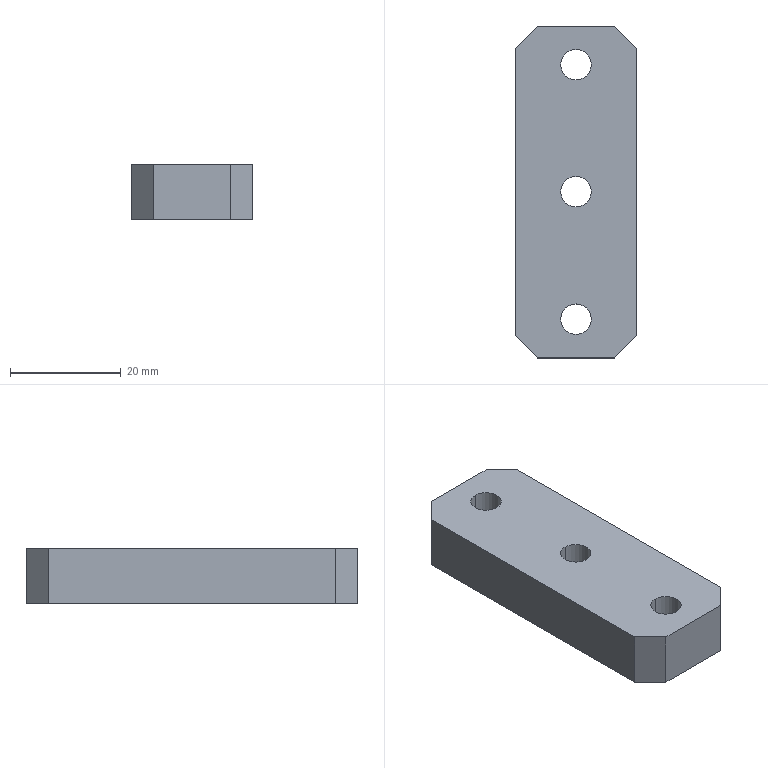Part | Creo | 1 solid | 25 faces | box 22 x 60 x 10 mm | volume 11319 mm3 | plane 13 | cylinder 12 | commonest cylinder face diameters 5.5 x6 9.5 x6
STEP:
#1=CARTESIAN_POINT('',(195.234,-215.142,-294.5));
#2=VERTEX_POINT('',#1);
#3=CARTESIAN_POINT('',(195.234,-163.142,-294.5));
#4=VERTEX_POINT('',#3);
#5=CARTESIAN_POINT('',(195.234,-215.142,-294.5));
#6=DIRECTION('',(0.,1.,0.));
#7=VECTOR('',#6,52.);
#8=LINE('',#5,#7);
#9=EDGE_CURVE('',#2,#4,#8,.T.);
#10=ORIENTED_EDGE('',*,*,#9,.F.);
#11=CARTESIAN_POINT('',(191.234,-219.142,-294.5));
#12=VERTEX_POINT('',#11);
#13=CARTESIAN_POINT('',(191.234,-219.142,-294.5));
#14=DIRECTION('',(0.7071,0.7071,0.));
#15=VECTOR('',#14,5.657);
#16=LINE('',#13,#15);
#17=EDGE_CURVE('',#12,#2,#16,.T.);
#18=ORIENTED_EDGE('',*,*,#17,.F.);
#19=CARTESIAN_POINT('',(177.234,-219.142,-294.5));
#20=VERTEX_POINT('',#19);
#21=CARTESIAN_POINT('',(191.234,-219.142,-294.5));
#22=DIRECTION('',(-1.,0.,0.));
#23=VECTOR('',#22,14.);
#24=LINE('',#21,#23);
#25=EDGE_CURVE('',#12,#20,#24,.T.);
#26=ORIENTED_EDGE('',*,*,#25,.T.);
#27=CARTESIAN_POINT('',(173.234,-215.142,-294.5));
#28=VERTEX_POINT('',#27);
#29=CARTESIAN_POINT('',(173.234,-215.142,-294.5));
#30=DIRECTION('',(0.7071,-0.7071,0.));
#31=VECTOR('',#30,5.657);
#32=LINE('',#29,#31);
#33=EDGE_CURVE('',#28,#20,#32,.T.);
#34=ORIENTED_EDGE('',*,*,#33,.F.);
#35=CARTESIAN_POINT('',(173.234,-163.142,-294.5));
#36=VERTEX_POINT('',#35);
#37=CARTESIAN_POINT('',(173.234,-163.142,-294.5));
#38=DIRECTION('',(0.,-1.,0.));
#39=VECTOR('',#38,52.);
#40=LINE('',#37,#39);
#41=EDGE_CURVE('',#36,#28,#40,.T.);
#42=ORIENTED_EDGE('',*,*,#41,.F.);
#43=CARTESIAN_POINT('',(177.234,-159.142,-294.5));
#44=VERTEX_POINT('',#43);
#45=CARTESIAN_POINT('',(177.234,-159.142,-294.5));
#46=DIRECTION('',(-0.7071,-0.7071,0.));
#47=VECTOR('',#46,5.657);
#48=LINE('',#45,#47);
#49=EDGE_CURVE('',#44,#36,#48,.T.);
#50=ORIENTED_EDGE('',*,*,#49,.F.);
#51=CARTESIAN_POINT('',(191.234,-159.142,-294.5));
#52=VERTEX_POINT('',#51);
#53=CARTESIAN_POINT('',(191.234,-159.142,-294.5));
#54=DIRECTION('',(-1.,0.,0.));
#55=VECTOR('',#54,14.);
#56=LINE('',#53,#55);
#57=EDGE_CURVE('',#52,#44,#56,.T.);
#58=ORIENTED_EDGE('',*,*,#57,.F.);
#59=CARTESIAN_POINT('',(195.234,-163.142,-294.5));
#60=DIRECTION('',(-0.7071,0.7071,0.));
#61=VECTOR('',#60,5.657);
#62=LINE('',#59,#61);
#63=EDGE_CURVE('',#4,#52,#62,.T.);
#64=ORIENTED_EDGE('',*,*,#63,.F.);
#65=EDGE_LOOP('',(#10,#18,#26,#34,#42,#50,#58,#64));
#66=FACE_OUTER_BOUND('',#65,.F.);
#67=CARTESIAN_POINT('',(184.234,-186.342,-294.5));
#68=VERTEX_POINT('',#67);
#69=CARTESIAN_POINT('',(184.234,-191.842,-294.5));
#70=VERTEX_POINT('',#69);
#71=CARTESIAN_POINT('',(184.234,-189.092,-294.5));
#72=DIRECTION('',(0.,0.,-1.));
#73=DIRECTION('',(0.,1.,0.));
#74=AXIS2_PLACEMENT_3D('',#71,#72,#73);
#75=CIRCLE('',#74,2.75);
#76=EDGE_CURVE('',#68,#70,#75,.T.);
#77=ORIENTED_EDGE('',*,*,#76,.F.);
#78=CARTESIAN_POINT('',(184.234,-189.092,-294.5));
#79=DIRECTION('',(0.,0.,-1.));
#80=DIRECTION('',(0.,-1.,0.));
#81=AXIS2_PLACEMENT_3D('',#78,#79,#80);
#82=CIRCLE('',#81,2.75);
#83=EDGE_CURVE('',#70,#68,#82,.T.);
#84=ORIENTED_EDGE('',*,*,#83,.F.);
#85=EDGE_LOOP('',(#77,#84));
#86=FACE_BOUND('',#85,.F.);
#87=CARTESIAN_POINT('',(184.234,-209.392,-294.5));
#88=VERTEX_POINT('',#87);
#89=CARTESIAN_POINT('',(184.234,-214.892,-294.5));
#90=VERTEX_POINT('',#89);
#91=CARTESIAN_POINT('',(184.234,-212.142,-294.5));
#92=DIRECTION('',(0.,0.,-1.));
#93=DIRECTION('',(0.,1.,0.));
#94=AXIS2_PLACEMENT_3D('',#91,#92,#93);
#95=CIRCLE('',#94,2.75);
#96=EDGE_CURVE('',#88,#90,#95,.T.);
#97=ORIENTED_EDGE('',*,*,#96,.F.);
#98=CARTESIAN_POINT('',(184.234,-212.142,-294.5));
#99=DIRECTION('',(0.,0.,-1.));
#100=DIRECTION('',(0.,-1.,0.));
#101=AXIS2_PLACEMENT_3D('',#98,#99,#100);
#102=CIRCLE('',#101,2.75);
#103=EDGE_CURVE('',#90,#88,#102,.T.);
#104=ORIENTED_EDGE('',*,*,#103,.F.);
#105=EDGE_LOOP('',(#97,#104));
#106=FACE_BOUND('',#105,.F.);
#107=CARTESIAN_POINT('',(184.234,-163.392,-294.5));
#108=VERTEX_POINT('',#107);
#109=CARTESIAN_POINT('',(184.234,-168.892,-294.5));
#110=VERTEX_POINT('',#109);
#111=CARTESIAN_POINT('',(184.234,-166.142,-294.5));
#112=DIRECTION('',(0.,0.,-1.));
#113=DIRECTION('',(0.,1.,0.));
#114=AXIS2_PLACEMENT_3D('',#111,#112,#113);
#115=CIRCLE('',#114,2.75);
#116=EDGE_CURVE('',#108,#110,#115,.T.);
#117=ORIENTED_EDGE('',*,*,#116,.F.);
#118=CARTESIAN_POINT('',(184.234,-166.142,-294.5));
#119=DIRECTION('',(0.,0.,-1.));
#120=DIRECTION('',(0.,-1.,0.));
#121=AXIS2_PLACEMENT_3D('',#118,#119,#120);
#122=CIRCLE('',#121,2.75);
#123=EDGE_CURVE('',#110,#108,#122,.T.);
#124=ORIENTED_EDGE('',*,*,#123,.F.);
#125=EDGE_LOOP('',(#117,#124));
#126=FACE_BOUND('',#125,.F.);
#127=CARTESIAN_POINT('',(174.234,-195.192,-294.5));
#128=DIRECTION('',(0.,0.,1.));
#129=DIRECTION('',(0.,-1.,0.));
#130=AXIS2_PLACEMENT_3D('',#127,#128,#129);
#131=PLANE('',#130);
#132=ADVANCED_FACE('',(#66,#86,#106,#126),#131,.T.);
#133=CARTESIAN_POINT('',(195.234,-163.142,-304.5));
#134=VERTEX_POINT('',#133);
#135=CARTESIAN_POINT('',(195.234,-215.142,-304.5));
#136=VERTEX_POINT('',#135);
#137=CARTESIAN_POINT('',(195.234,-163.142,-304.5));
#138=DIRECTION('',(0.,-1.,0.));
#139=VECTOR('',#138,52.);
#140=LINE('',#137,#139);
#141=EDGE_CURVE('',#134,#136,#140,.T.);
#142=ORIENTED_EDGE('',*,*,#141,.T.);
#143=CARTESIAN_POINT('',(195.234,-215.142,-294.5));
#144=DIRECTION('',(0.,0.,-1.));
#145=VECTOR('',#144,10.);
#146=LINE('',#143,#145);
#147=EDGE_CURVE('',#2,#136,#146,.T.);
#148=ORIENTED_EDGE('',*,*,#147,.F.);
#149=ORIENTED_EDGE('',*,*,#9,.T.);
#150=CARTESIAN_POINT('',(195.234,-163.142,-304.5));
#151=DIRECTION('',(0.,0.,1.));
#152=VECTOR('',#151,10.);
#153=LINE('',#150,#152);
#154=EDGE_CURVE('',#134,#4,#153,.T.);
#155=ORIENTED_EDGE('',*,*,#154,.F.);
#156=EDGE_LOOP('',(#142,#148,#149,#155));
#157=FACE_OUTER_BOUND('',#156,.F.);
#158=CARTESIAN_POINT('',(195.234,-212.942,-299.5));
#159=DIRECTION('',(-1.,0.,0.));
#160=DIRECTION('',(0.,0.,1.));
#161=AXIS2_PLACEMENT_3D('',#158,#159,#160);
#162=PLANE('',#161);
#163=ADVANCED_FACE('',(#157),#162,.F.);
#164=CARTESIAN_POINT('',(173.234,-215.142,-304.5));
#165=VERTEX_POINT('',#164);
#166=CARTESIAN_POINT('',(173.234,-163.142,-304.5));
#167=VERTEX_POINT('',#166);
#168=CARTESIAN_POINT('',(173.234,-215.142,-304.5));
#169=DIRECTION('',(0.,1.,0.));
#170=VECTOR('',#169,52.);
#171=LINE('',#168,#170);
#172=EDGE_CURVE('',#165,#167,#171,.T.);
#173=ORIENTED_EDGE('',*,*,#172,.F.);
#174=CARTESIAN_POINT('',(177.234,-219.142,-304.5));
#175=VERTEX_POINT('',#174);
#176=CARTESIAN_POINT('',(177.234,-219.142,-304.5));
#177=DIRECTION('',(-0.7071,0.7071,0.));
#178=VECTOR('',#177,5.657);
#179=LINE('',#176,#178);
#180=EDGE_CURVE('',#175,#165,#179,.T.);
#181=ORIENTED_EDGE('',*,*,#180,.F.);
#182=CARTESIAN_POINT('',(191.234,-219.142,-304.5));
#183=VERTEX_POINT('',#182);
#184=CARTESIAN_POINT('',(177.234,-219.142,-304.5));
#185=DIRECTION('',(1.,0.,0.));
#186=VECTOR('',#185,14.);
#187=LINE('',#184,#186);
#188=EDGE_CURVE('',#175,#183,#187,.T.);
#189=ORIENTED_EDGE('',*,*,#188,.T.);
#190=CARTESIAN_POINT('',(195.234,-215.142,-304.5));
#191=DIRECTION('',(-0.7071,-0.7071,0.));
#192=VECTOR('',#191,5.657);
#193=LINE('',#190,#192);
#194=EDGE_CURVE('',#136,#183,#193,.T.);
#195=ORIENTED_EDGE('',*,*,#194,.F.);
#196=ORIENTED_EDGE('',*,*,#141,.F.);
#197=CARTESIAN_POINT('',(191.234,-159.142,-304.5));
#198=VERTEX_POINT('',#197);
#199=CARTESIAN_POINT('',(191.234,-159.142,-304.5));
#200=DIRECTION('',(0.7071,-0.7071,0.));
#201=VECTOR('',#200,5.657);
#202=LINE('',#199,#201);
#203=EDGE_CURVE('',#198,#134,#202,.T.);
#204=ORIENTED_EDGE('',*,*,#203,.F.);
#205=CARTESIAN_POINT('',(177.234,-159.142,-304.5));
#206=VERTEX_POINT('',#205);
#207=CARTESIAN_POINT('',(177.234,-159.142,-304.5));
#208=DIRECTION('',(1.,0.,0.));
#209=VECTOR('',#208,14.);
#210=LINE('',#207,#209);
#211=EDGE_CURVE('',#206,#198,#210,.T.);
#212=ORIENTED_EDGE('',*,*,#211,.F.);
#213=CARTESIAN_POINT('',(173.234,-163.142,-304.5));
#214=DIRECTION('',(0.7071,0.7071,0.));
#215=VECTOR('',#214,5.657);
#216=LINE('',#213,#215);
#217=EDGE_CURVE('',#167,#206,#216,.T.);
#218=ORIENTED_EDGE('',*,*,#217,.F.);
#219=EDGE_LOOP('',(#173,#181,#189,#195,#196,#204,#212,#218));
#220=FACE_OUTER_BOUND('',#219,.F.);
#221=CARTESIAN_POINT('',(184.234,-184.342,-304.5));
#222=VERTEX_POINT('',#221);
#223=CARTESIAN_POINT('',(184.234,-193.842,-304.5));
#224=VERTEX_POINT('',#223);
#225=CARTESIAN_POINT('',(184.234,-189.092,-304.5));
#226=DIRECTION('',(0.,0.,1.));
#227=DIRECTION('',(0.,1.,0.));
#228=AXIS2_PLACEMENT_3D('',#225,#226,#227);
#229=CIRCLE('',#228,4.75);
#230=EDGE_CURVE('',#222,#224,#229,.T.);
#231=ORIENTED_EDGE('',*,*,#230,.F.);
#232=CARTESIAN_POINT('',(184.234,-189.092,-304.5));
#233=DIRECTION('',(0.,0.,1.));
#234=DIRECTION('',(0.,-1.,0.));
#235=AXIS2_PLACEMENT_3D('',#232,#233,#234);
#236=CIRCLE('',#235,4.75);
#237=EDGE_CURVE('',#224,#222,#236,.T.);
#238=ORIENTED_EDGE('',*,*,#237,.F.);
#239=EDGE_LOOP('',(#231,#238));
#240=FACE_BOUND('',#239,.F.);
#241=CARTESIAN_POINT('',(184.234,-207.392,-304.5));
#242=VERTEX_POINT('',#241);
#243=CARTESIAN_POINT('',(184.234,-216.892,-304.5));
#244=VERTEX_POINT('',#243);
#245=CARTESIAN_POINT('',(184.234,-212.142,-304.5));
#246=DIRECTION('',(0.,0.,1.));
#247=DIRECTION('',(0.,1.,0.));
#248=AXIS2_PLACEMENT_3D('',#245,#246,#247);
#249=CIRCLE('',#248,4.75);
#250=EDGE_CURVE('',#242,#244,#249,.T.);
#251=ORIENTED_EDGE('',*,*,#250,.F.);
#252=CARTESIAN_POINT('',(184.234,-212.142,-304.5));
#253=DIRECTION('',(0.,0.,1.));
#254=DIRECTION('',(0.,-1.,0.));
#255=AXIS2_PLACEMENT_3D('',#252,#253,#254);
#256=CIRCLE('',#255,4.75);
#257=EDGE_CURVE('',#244,#242,#256,.T.);
#258=ORIENTED_EDGE('',*,*,#257,.F.);
#259=EDGE_LOOP('',(#251,#258));
#260=FACE_BOUND('',#259,.F.);
#261=CARTESIAN_POINT('',(184.234,-161.392,-304.5));
#262=VERTEX_POINT('',#261);
#263=CARTESIAN_POINT('',(184.234,-170.892,-304.5));
#264=VERTEX_POINT('',#263);
#265=CARTESIAN_POINT('',(184.234,-166.142,-304.5));
#266=DIRECTION('',(0.,0.,1.));
#267=DIRECTION('',(0.,1.,0.));
#268=AXIS2_PLACEMENT_3D('',#265,#266,#267);
#269=CIRCLE('',#268,4.75);
#270=EDGE_CURVE('',#262,#264,#269,.T.);
#271=ORIENTED_EDGE('',*,*,#270,.F.);
#272=CARTESIAN_POINT('',(184.234,-166.142,-304.5));
#273=DIRECTION('',(0.,0.,1.));
#274=DIRECTION('',(0.,-1.,0.));
#275=AXIS2_PLACEMENT_3D('',#272,#273,#274);
#276=CIRCLE('',#275,4.75);
#277=EDGE_CURVE('',#264,#262,#276,.T.);
#278=ORIENTED_EDGE('',*,*,#277,.F.);
#279=EDGE_LOOP('',(#271,#278));
#280=FACE_BOUND('',#279,.F.);
#281=CARTESIAN_POINT('',(174.234,-195.192,-304.5));
#282=DIRECTION('',(0.,0.,-1.));
#283=DIRECTION('',(0.,1.,0.));
#284=AXIS2_PLACEMENT_3D('',#281,#282,#283);
#285=PLANE('',#284);
#286=ADVANCED_FACE('',(#220,#240,#260,#280),#285,.T.);
#287=ORIENTED_EDGE('',*,*,#41,.T.);
#288=CARTESIAN_POINT('',(173.234,-215.142,-304.5));
#289=DIRECTION('',(0.,0.,1.));
#290=VECTOR('',#289,10.);
#291=LINE('',#288,#290);
#292=EDGE_CURVE('',#165,#28,#291,.T.);
#293=ORIENTED_EDGE('',*,*,#292,.F.);
#294=ORIENTED_EDGE('',*,*,#172,.T.);
#295=CARTESIAN_POINT('',(173.234,-163.142,-294.5));
#296=DIRECTION('',(0.,0.,-1.));
#297=VECTOR('',#296,10.);
#298=LINE('',#295,#297);
#299=EDGE_CURVE('',#36,#167,#298,.T.);
#300=ORIENTED_EDGE('',*,*,#299,.F.);
#301=EDGE_LOOP('',(#287,#293,#294,#300));
#302=FACE_OUTER_BOUND('',#301,.F.);
#303=CARTESIAN_POINT('',(173.234,-190.442,-299.5));
#304=DIRECTION('',(1.,0.,0.));
#305=DIRECTION('',(0.,0.,1.));
#306=AXIS2_PLACEMENT_3D('',#303,#304,#305);
#307=PLANE('',#306);
#308=ADVANCED_FACE('',(#302),#307,.F.);
#309=ORIENTED_EDGE('',*,*,#180,.T.);
#310=ORIENTED_EDGE('',*,*,#292,.T.);
#311=ORIENTED_EDGE('',*,*,#33,.T.);
#312=CARTESIAN_POINT('',(177.234,-219.142,-294.5));
#313=DIRECTION('',(0.,0.,-1.));
#314=VECTOR('',#313,10.);
#315=LINE('',#312,#314);
#316=EDGE_CURVE('',#20,#175,#315,.T.);
#317=ORIENTED_EDGE('',*,*,#316,.T.);
#318=EDGE_LOOP('',(#309,#310,#311,#317));
#319=FACE_OUTER_BOUND('',#318,.F.);
#320=CARTESIAN_POINT('',(177.234,-219.142,-299.5));
#321=DIRECTION('',(0.7071,0.7071,0.));
#322=DIRECTION('',(0.7071,-0.7071,0.));
#323=AXIS2_PLACEMENT_3D('',#320,#321,#322);
#324=PLANE('',#323);
#325=ADVANCED_FACE('',(#319),#324,.F.);
#326=ORIENTED_EDGE('',*,*,#25,.F.);
#327=CARTESIAN_POINT('',(191.234,-219.142,-304.5));
#328=DIRECTION('',(0.,0.,1.));
#329=VECTOR('',#328,10.);
#330=LINE('',#327,#329);
#331=EDGE_CURVE('',#183,#12,#330,.T.);
#332=ORIENTED_EDGE('',*,*,#331,.F.);
#333=ORIENTED_EDGE('',*,*,#188,.F.);
#334=ORIENTED_EDGE('',*,*,#316,.F.);
#335=EDGE_LOOP('',(#326,#332,#333,#334));
#336=FACE_OUTER_BOUND('',#335,.F.);
#337=CARTESIAN_POINT('',(172.234,-219.142,-299.5));
#338=DIRECTION('',(0.,1.,0.));
#339=DIRECTION('',(0.,0.,-1.));
#340=AXIS2_PLACEMENT_3D('',#337,#338,#339);
#341=PLANE('',#340);
#342=ADVANCED_FACE('',(#336),#341,.F.);
#343=ORIENTED_EDGE('',*,*,#194,.T.);
#344=ORIENTED_EDGE('',*,*,#331,.T.);
#345=ORIENTED_EDGE('',*,*,#17,.T.);
#346=ORIENTED_EDGE('',*,*,#147,.T.);
#347=EDGE_LOOP('',(#343,#344,#345,#346));
#348=FACE_OUTER_BOUND('',#347,.F.);
#349=CARTESIAN_POINT('',(195.234,-215.142,-299.5));
#350=DIRECTION('',(-0.7071,0.7071,0.));
#351=DIRECTION('',(0.7071,0.7071,0.));
#352=AXIS2_PLACEMENT_3D('',#349,#350,#351);
#353=PLANE('',#352);
#354=ADVANCED_FACE('',(#348),#353,.F.);
#355=ORIENTED_EDGE('',*,*,#217,.T.);
#356=CARTESIAN_POINT('',(177.234,-159.142,-304.5));
#357=DIRECTION('',(0.,0.,1.));
#358=VECTOR('',#357,10.);
#359=LINE('',#356,#358);
#360=EDGE_CURVE('',#206,#44,#359,.T.);
#361=ORIENTED_EDGE('',*,*,#360,.T.);
#362=ORIENTED_EDGE('',*,*,#49,.T.);
#363=ORIENTED_EDGE('',*,*,#299,.T.);
#364=EDGE_LOOP('',(#355,#361,#362,#363));
#365=FACE_OUTER_BOUND('',#364,.F.);
#366=CARTESIAN_POINT('',(173.234,-163.142,-299.5));
#367=DIRECTION('',(0.7071,-0.7071,0.));
#368=DIRECTION('',(-0.7071,-0.7071,0.));
#369=AXIS2_PLACEMENT_3D('',#366,#367,#368);
#370=PLANE('',#369);
#371=ADVANCED_FACE('',(#365),#370,.F.);
#372=ORIENTED_EDGE('',*,*,#57,.T.);
#373=ORIENTED_EDGE('',*,*,#360,.F.);
#374=ORIENTED_EDGE('',*,*,#211,.T.);
#375=CARTESIAN_POINT('',(191.234,-159.142,-294.5));
#376=DIRECTION('',(0.,0.,-1.));
#377=VECTOR('',#376,10.);
#378=LINE('',#375,#377);
#379=EDGE_CURVE('',#52,#198,#378,.T.);
#380=ORIENTED_EDGE('',*,*,#379,.F.);
#381=EDGE_LOOP('',(#372,#373,#374,#380));
#382=FACE_OUTER_BOUND('',#381,.F.);
#383=CARTESIAN_POINT('',(172.234,-159.142,-299.5));
#384=DIRECTION('',(0.,-1.,0.));
#385=DIRECTION('',(0.,0.,-1.));
#386=AXIS2_PLACEMENT_3D('',#383,#384,#385);
#387=PLANE('',#386);
#388=ADVANCED_FACE('',(#382),#387,.F.);
#389=ORIENTED_EDGE('',*,*,#203,.T.);
#390=ORIENTED_EDGE('',*,*,#154,.T.);
#391=ORIENTED_EDGE('',*,*,#63,.T.);
#392=ORIENTED_EDGE('',*,*,#379,.T.);
#393=EDGE_LOOP('',(#389,#390,#391,#392));
#394=FACE_OUTER_BOUND('',#393,.F.);
#395=CARTESIAN_POINT('',(191.234,-159.142,-299.5));
#396=DIRECTION('',(-0.7071,-0.7071,0.));
#397=DIRECTION('',(-0.7071,0.7071,0.));
#398=AXIS2_PLACEMENT_3D('',#395,#396,#397);
#399=PLANE('',#398);
#400=ADVANCED_FACE('',(#394),#399,.F.);
#401=ORIENTED_EDGE('',*,*,#230,.T.);
#402=CARTESIAN_POINT('',(184.234,-193.842,-298.5));
#403=VERTEX_POINT('',#402);
#404=CARTESIAN_POINT('',(184.234,-193.842,-298.5));
#405=DIRECTION('',(0.,0.,-1.));
#406=VECTOR('',#405,6.);
#407=LINE('',#404,#406);
#408=EDGE_CURVE('',#403,#224,#407,.T.);
#409=ORIENTED_EDGE('',*,*,#408,.F.);
#410=CARTESIAN_POINT('',(184.234,-184.342,-298.5));
#411=VERTEX_POINT('',#410);
#412=CARTESIAN_POINT('',(184.234,-189.092,-298.5));
#413=DIRECTION('',(0.,0.,-1.));
#414=DIRECTION('',(0.,-1.,0.));
#415=AXIS2_PLACEMENT_3D('',#412,#413,#414);
#416=CIRCLE('',#415,4.75);
#417=EDGE_CURVE('',#403,#411,#416,.T.);
#418=ORIENTED_EDGE('',*,*,#417,.T.);
#419=CARTESIAN_POINT('',(184.234,-184.342,-298.5));
#420=DIRECTION('',(0.,0.,-1.));
#421=VECTOR('',#420,6.);
#422=LINE('',#419,#421);
#423=EDGE_CURVE('',#411,#222,#422,.T.);
#424=ORIENTED_EDGE('',*,*,#423,.T.);
#425=EDGE_LOOP('',(#401,#409,#418,#424));
#426=FACE_OUTER_BOUND('',#425,.F.);
#427=CARTESIAN_POINT('',(184.234,-189.092,-298.5));
#428=DIRECTION('',(0.,0.,-1.));
#429=DIRECTION('',(0.,1.,0.));
#430=AXIS2_PLACEMENT_3D('',#427,#428,#429);
#431=CYLINDRICAL_SURFACE('',#430,4.75);
#432=ADVANCED_FACE('',(#426),#431,.F.);
#433=ORIENTED_EDGE('',*,*,#237,.T.);
#434=ORIENTED_EDGE('',*,*,#423,.F.);
#435=CARTESIAN_POINT('',(184.234,-189.092,-298.5));
#436=DIRECTION('',(0.,0.,-1.));
#437=DIRECTION('',(0.,1.,0.));
#438=AXIS2_PLACEMENT_3D('',#435,#436,#437);
#439=CIRCLE('',#438,4.75);
#440=EDGE_CURVE('',#411,#403,#439,.T.);
#441=ORIENTED_EDGE('',*,*,#440,.T.);
#442=ORIENTED_EDGE('',*,*,#408,.T.);
#443=EDGE_LOOP('',(#433,#434,#441,#442));
#444=FACE_OUTER_BOUND('',#443,.F.);
#445=CARTESIAN_POINT('',(184.234,-189.092,-298.5));
#446=DIRECTION('',(0.,0.,-1.));
#447=DIRECTION('',(0.,1.,0.));
#448=AXIS2_PLACEMENT_3D('',#445,#446,#447);
#449=CYLINDRICAL_SURFACE('',#448,4.75);
#450=ADVANCED_FACE('',(#444),#449,.F.);
#451=ORIENTED_EDGE('',*,*,#440,.F.);
#452=ORIENTED_EDGE('',*,*,#417,.F.);
#453=EDGE_LOOP('',(#451,#452));
#454=FACE_OUTER_BOUND('',#453,.F.);
#455=CARTESIAN_POINT('',(184.234,-186.342,-298.5));
#456=VERTEX_POINT('',#455);
#457=CARTESIAN_POINT('',(184.234,-191.842,-298.5));
#458=VERTEX_POINT('',#457);
#459=CARTESIAN_POINT('',(184.234,-189.092,-298.5));
#460=DIRECTION('',(0.,0.,1.));
#461=DIRECTION('',(0.,1.,0.));
#462=AXIS2_PLACEMENT_3D('',#459,#460,#461);
#463=CIRCLE('',#462,2.75);
#464=EDGE_CURVE('',#456,#458,#463,.T.);
#465=ORIENTED_EDGE('',*,*,#464,.F.);
#466=CARTESIAN_POINT('',(184.234,-189.092,-298.5));
#467=DIRECTION('',(0.,0.,1.));
#468=DIRECTION('',(0.,-1.,0.));
#469=AXIS2_PLACEMENT_3D('',#466,#467,#468);
#470=CIRCLE('',#469,2.75);
#471=EDGE_CURVE('',#458,#456,#470,.T.);
#472=ORIENTED_EDGE('',*,*,#471,.F.);
#473=EDGE_LOOP('',(#465,#472));
#474=FACE_BOUND('',#473,.F.);
#475=CARTESIAN_POINT('',(184.234,-189.092,-298.5));
#476=DIRECTION('',(0.,0.,1.));
#477=DIRECTION('',(0.,-1.,0.));
#478=AXIS2_PLACEMENT_3D('',#475,#476,#477);
#479=PLANE('',#478);
#480=ADVANCED_FACE('',(#454,#474),#479,.F.);
#481=ORIENTED_EDGE('',*,*,#464,.T.);
#482=CARTESIAN_POINT('',(184.234,-191.842,-294.5));
#483=DIRECTION('',(0.,0.,-1.));
#484=VECTOR('',#483,4.);
#485=LINE('',#482,#484);
#486=EDGE_CURVE('',#70,#458,#485,.T.);
#487=ORIENTED_EDGE('',*,*,#486,.F.);
#488=ORIENTED_EDGE('',*,*,#83,.T.);
#489=CARTESIAN_POINT('',(184.234,-186.342,-294.5));
#490=DIRECTION('',(0.,0.,-1.));
#491=VECTOR('',#490,4.);
#492=LINE('',#489,#491);
#493=EDGE_CURVE('',#68,#456,#492,.T.);
#494=ORIENTED_EDGE('',*,*,#493,.T.);
#495=EDGE_LOOP('',(#481,#487,#488,#494));
#496=FACE_OUTER_BOUND('',#495,.F.);
#497=CARTESIAN_POINT('',(184.234,-189.092,-294.5));
#498=DIRECTION('',(0.,0.,-1.));
#499=DIRECTION('',(0.,1.,0.));
#500=AXIS2_PLACEMENT_3D('',#497,#498,#499);
#501=CYLINDRICAL_SURFACE('',#500,2.75);
#502=ADVANCED_FACE('',(#496),#501,.F.);
#503=ORIENTED_EDGE('',*,*,#471,.T.);
#504=ORIENTED_EDGE('',*,*,#493,.F.);
#505=ORIENTED_EDGE('',*,*,#76,.T.);
#506=ORIENTED_EDGE('',*,*,#486,.T.);
#507=EDGE_LOOP('',(#503,#504,#505,#506));
#508=FACE_OUTER_BOUND('',#507,.F.);
#509=CARTESIAN_POINT('',(184.234,-189.092,-294.5));
#510=DIRECTION('',(0.,0.,-1.));
#511=DIRECTION('',(0.,1.,0.));
#512=AXIS2_PLACEMENT_3D('',#509,#510,#511);
#513=CYLINDRICAL_SURFACE('',#512,2.75);
#514=ADVANCED_FACE('',(#508),#513,.F.);
#515=ORIENTED_EDGE('',*,*,#250,.T.);
#516=CARTESIAN_POINT('',(184.234,-216.892,-298.5));
#517=VERTEX_POINT('',#516);
#518=CARTESIAN_POINT('',(184.234,-216.892,-298.5));
#519=DIRECTION('',(0.,0.,-1.));
#520=VECTOR('',#519,6.);
#521=LINE('',#518,#520);
#522=EDGE_CURVE('',#517,#244,#521,.T.);
#523=ORIENTED_EDGE('',*,*,#522,.F.);
#524=CARTESIAN_POINT('',(184.234,-207.392,-298.5));
#525=VERTEX_POINT('',#524);
#526=CARTESIAN_POINT('',(184.234,-212.142,-298.5));
#527=DIRECTION('',(0.,0.,-1.));
#528=DIRECTION('',(0.,-1.,0.));
#529=AXIS2_PLACEMENT_3D('',#526,#527,#528);
#530=CIRCLE('',#529,4.75);
#531=EDGE_CURVE('',#517,#525,#530,.T.);
#532=ORIENTED_EDGE('',*,*,#531,.T.);
#533=CARTESIAN_POINT('',(184.234,-207.392,-298.5));
#534=DIRECTION('',(0.,0.,-1.));
#535=VECTOR('',#534,6.);
#536=LINE('',#533,#535);
#537=EDGE_CURVE('',#525,#242,#536,.T.);
#538=ORIENTED_EDGE('',*,*,#537,.T.);
#539=EDGE_LOOP('',(#515,#523,#532,#538));
#540=FACE_OUTER_BOUND('',#539,.F.);
#541=CARTESIAN_POINT('',(184.234,-212.142,-298.5));
#542=DIRECTION('',(0.,0.,-1.));
#543=DIRECTION('',(0.,1.,0.));
#544=AXIS2_PLACEMENT_3D('',#541,#542,#543);
#545=CYLINDRICAL_SURFACE('',#544,4.75);
#546=ADVANCED_FACE('',(#540),#545,.F.);
#547=ORIENTED_EDGE('',*,*,#257,.T.);
#548=ORIENTED_EDGE('',*,*,#537,.F.);
#549=CARTESIAN_POINT('',(184.234,-212.142,-298.5));
#550=DIRECTION('',(0.,0.,-1.));
#551=DIRECTION('',(0.,1.,0.));
#552=AXIS2_PLACEMENT_3D('',#549,#550,#551);
#553=CIRCLE('',#552,4.75);
#554=EDGE_CURVE('',#525,#517,#553,.T.);
#555=ORIENTED_EDGE('',*,*,#554,.T.);
#556=ORIENTED_EDGE('',*,*,#522,.T.);
#557=EDGE_LOOP('',(#547,#548,#555,#556));
#558=FACE_OUTER_BOUND('',#557,.F.);
#559=CARTESIAN_POINT('',(184.234,-212.142,-298.5));
#560=DIRECTION('',(0.,0.,-1.));
#561=DIRECTION('',(0.,1.,0.));
#562=AXIS2_PLACEMENT_3D('',#559,#560,#561);
#563=CYLINDRICAL_SURFACE('',#562,4.75);
#564=ADVANCED_FACE('',(#558),#563,.F.);
#565=ORIENTED_EDGE('',*,*,#554,.F.);
#566=ORIENTED_EDGE('',*,*,#531,.F.);
#567=EDGE_LOOP('',(#565,#566));
#568=FACE_OUTER_BOUND('',#567,.F.);
#569=CARTESIAN_POINT('',(184.234,-209.392,-298.5));
#570=VERTEX_POINT('',#569);
#571=CARTESIAN_POINT('',(184.234,-214.892,-298.5));
#572=VERTEX_POINT('',#571);
#573=CARTESIAN_POINT('',(184.234,-212.142,-298.5));
#574=DIRECTION('',(0.,0.,1.));
#575=DIRECTION('',(0.,1.,0.));
#576=AXIS2_PLACEMENT_3D('',#573,#574,#575);
#577=CIRCLE('',#576,2.75);
#578=EDGE_CURVE('',#570,#572,#577,.T.);
#579=ORIENTED_EDGE('',*,*,#578,.F.);
#580=CARTESIAN_POINT('',(184.234,-212.142,-298.5));
#581=DIRECTION('',(0.,0.,1.));
#582=DIRECTION('',(0.,-1.,0.));
#583=AXIS2_PLACEMENT_3D('',#580,#581,#582);
#584=CIRCLE('',#583,2.75);
#585=EDGE_CURVE('',#572,#570,#584,.T.);
#586=ORIENTED_EDGE('',*,*,#585,.F.);
#587=EDGE_LOOP('',(#579,#586));
#588=FACE_BOUND('',#587,.F.);
#589=CARTESIAN_POINT('',(184.234,-212.142,-298.5));
#590=DIRECTION('',(0.,0.,1.));
#591=DIRECTION('',(0.,-1.,0.));
#592=AXIS2_PLACEMENT_3D('',#589,#590,#591);
#593=PLANE('',#592);
#594=ADVANCED_FACE('',(#568,#588),#593,.F.);
#595=ORIENTED_EDGE('',*,*,#578,.T.);
#596=CARTESIAN_POINT('',(184.234,-214.892,-294.5));
#597=DIRECTION('',(0.,0.,-1.));
#598=VECTOR('',#597,4.);
#599=LINE('',#596,#598);
#600=EDGE_CURVE('',#90,#572,#599,.T.);
#601=ORIENTED_EDGE('',*,*,#600,.F.);
#602=ORIENTED_EDGE('',*,*,#103,.T.);
#603=CARTESIAN_POINT('',(184.234,-209.392,-294.5));
#604=DIRECTION('',(0.,0.,-1.));
#605=VECTOR('',#604,4.);
#606=LINE('',#603,#605);
#607=EDGE_CURVE('',#88,#570,#606,.T.);
#608=ORIENTED_EDGE('',*,*,#607,.T.);
#609=EDGE_LOOP('',(#595,#601,#602,#608));
#610=FACE_OUTER_BOUND('',#609,.F.);
#611=CARTESIAN_POINT('',(184.234,-212.142,-294.5));
#612=DIRECTION('',(0.,0.,-1.));
#613=DIRECTION('',(0.,1.,0.));
#614=AXIS2_PLACEMENT_3D('',#611,#612,#613);
#615=CYLINDRICAL_SURFACE('',#614,2.75);
#616=ADVANCED_FACE('',(#610),#615,.F.);
#617=ORIENTED_EDGE('',*,*,#585,.T.);
#618=ORIENTED_EDGE('',*,*,#607,.F.);
#619=ORIENTED_EDGE('',*,*,#96,.T.);
#620=ORIENTED_EDGE('',*,*,#600,.T.);
#621=EDGE_LOOP('',(#617,#618,#619,#620));
#622=FACE_OUTER_BOUND('',#621,.F.);
#623=CARTESIAN_POINT('',(184.234,-212.142,-294.5));
#624=DIRECTION('',(0.,0.,-1.));
#625=DIRECTION('',(0.,1.,0.));
#626=AXIS2_PLACEMENT_3D('',#623,#624,#625);
#627=CYLINDRICAL_SURFACE('',#626,2.75);
#628=ADVANCED_FACE('',(#622),#627,.F.);
#629=ORIENTED_EDGE('',*,*,#270,.T.);
#630=CARTESIAN_POINT('',(184.234,-170.892,-298.5));
#631=VERTEX_POINT('',#630);
#632=CARTESIAN_POINT('',(184.234,-170.892,-298.5));
#633=DIRECTION('',(0.,0.,-1.));
#634=VECTOR('',#633,6.);
#635=LINE('',#632,#634);
#636=EDGE_CURVE('',#631,#264,#635,.T.);
#637=ORIENTED_EDGE('',*,*,#636,.F.);
#638=CARTESIAN_POINT('',(184.234,-161.392,-298.5));
#639=VERTEX_POINT('',#638);
#640=CARTESIAN_POINT('',(184.234,-166.142,-298.5));
#641=DIRECTION('',(0.,0.,-1.));
#642=DIRECTION('',(0.,-1.,0.));
#643=AXIS2_PLACEMENT_3D('',#640,#641,#642);
#644=CIRCLE('',#643,4.75);
#645=EDGE_CURVE('',#631,#639,#644,.T.);
#646=ORIENTED_EDGE('',*,*,#645,.T.);
#647=CARTESIAN_POINT('',(184.234,-161.392,-298.5));
#648=DIRECTION('',(0.,0.,-1.));
#649=VECTOR('',#648,6.);
#650=LINE('',#647,#649);
#651=EDGE_CURVE('',#639,#262,#650,.T.);
#652=ORIENTED_EDGE('',*,*,#651,.T.);
#653=EDGE_LOOP('',(#629,#637,#646,#652));
#654=FACE_OUTER_BOUND('',#653,.F.);
#655=CARTESIAN_POINT('',(184.234,-166.142,-298.5));
#656=DIRECTION('',(0.,0.,-1.));
#657=DIRECTION('',(0.,1.,0.));
#658=AXIS2_PLACEMENT_3D('',#655,#656,#657);
#659=CYLINDRICAL_SURFACE('',#658,4.75);
#660=ADVANCED_FACE('',(#654),#659,.F.);
#661=ORIENTED_EDGE('',*,*,#277,.T.);
#662=ORIENTED_EDGE('',*,*,#651,.F.);
#663=CARTESIAN_POINT('',(184.234,-166.142,-298.5));
#664=DIRECTION('',(0.,0.,-1.));
#665=DIRECTION('',(0.,1.,0.));
#666=AXIS2_PLACEMENT_3D('',#663,#664,#665);
#667=CIRCLE('',#666,4.75);
#668=EDGE_CURVE('',#639,#631,#667,.T.);
#669=ORIENTED_EDGE('',*,*,#668,.T.);
#670=ORIENTED_EDGE('',*,*,#636,.T.);
#671=EDGE_LOOP('',(#661,#662,#669,#670));
#672=FACE_OUTER_BOUND('',#671,.F.);
#673=CARTESIAN_POINT('',(184.234,-166.142,-298.5));
#674=DIRECTION('',(0.,0.,-1.));
#675=DIRECTION('',(0.,1.,0.));
#676=AXIS2_PLACEMENT_3D('',#673,#674,#675);
#677=CYLINDRICAL_SURFACE('',#676,4.75);
#678=ADVANCED_FACE('',(#672),#677,.F.);
#679=ORIENTED_EDGE('',*,*,#668,.F.);
#680=ORIENTED_EDGE('',*,*,#645,.F.);
#681=EDGE_LOOP('',(#679,#680));
#682=FACE_OUTER_BOUND('',#681,.F.);
#683=CARTESIAN_POINT('',(184.234,-163.392,-298.5));
#684=VERTEX_POINT('',#683);
#685=CARTESIAN_POINT('',(184.234,-168.892,-298.5));
#686=VERTEX_POINT('',#685);
#687=CARTESIAN_POINT('',(184.234,-166.142,-298.5));
#688=DIRECTION('',(0.,0.,1.));
#689=DIRECTION('',(0.,1.,0.));
#690=AXIS2_PLACEMENT_3D('',#687,#688,#689);
#691=CIRCLE('',#690,2.75);
#692=EDGE_CURVE('',#684,#686,#691,.T.);
#693=ORIENTED_EDGE('',*,*,#692,.F.);
#694=CARTESIAN_POINT('',(184.234,-166.142,-298.5));
#695=DIRECTION('',(0.,0.,1.));
#696=DIRECTION('',(0.,-1.,0.));
#697=AXIS2_PLACEMENT_3D('',#694,#695,#696);
#698=CIRCLE('',#697,2.75);
#699=EDGE_CURVE('',#686,#684,#698,.T.);
#700=ORIENTED_EDGE('',*,*,#699,.F.);
#701=EDGE_LOOP('',(#693,#700));
#702=FACE_BOUND('',#701,.F.);
#703=CARTESIAN_POINT('',(184.234,-166.142,-298.5));
#704=DIRECTION('',(0.,0.,1.));
#705=DIRECTION('',(0.,-1.,0.));
#706=AXIS2_PLACEMENT_3D('',#703,#704,#705);
#707=PLANE('',#706);
#708=ADVANCED_FACE('',(#682,#702),#707,.F.);
#709=ORIENTED_EDGE('',*,*,#692,.T.);
#710=CARTESIAN_POINT('',(184.234,-168.892,-294.5));
#711=DIRECTION('',(0.,0.,-1.));
#712=VECTOR('',#711,4.);
#713=LINE('',#710,#712);
#714=EDGE_CURVE('',#110,#686,#713,.T.);
#715=ORIENTED_EDGE('',*,*,#714,.F.);
#716=ORIENTED_EDGE('',*,*,#123,.T.);
#717=CARTESIAN_POINT('',(184.234,-163.392,-294.5));
#718=DIRECTION('',(0.,0.,-1.));
#719=VECTOR('',#718,4.);
#720=LINE('',#717,#719);
#721=EDGE_CURVE('',#108,#684,#720,.T.);
#722=ORIENTED_EDGE('',*,*,#721,.T.);
#723=EDGE_LOOP('',(#709,#715,#716,#722));
#724=FACE_OUTER_BOUND('',#723,.F.);
#725=CARTESIAN_POINT('',(184.234,-166.142,-294.5));
#726=DIRECTION('',(0.,0.,-1.));
#727=DIRECTION('',(0.,1.,0.));
#728=AXIS2_PLACEMENT_3D('',#725,#726,#727);
#729=CYLINDRICAL_SURFACE('',#728,2.75);
#730=ADVANCED_FACE('',(#724),#729,.F.);
#731=ORIENTED_EDGE('',*,*,#699,.T.);
#732=ORIENTED_EDGE('',*,*,#721,.F.);
#733=ORIENTED_EDGE('',*,*,#116,.T.);
#734=ORIENTED_EDGE('',*,*,#714,.T.);
#735=EDGE_LOOP('',(#731,#732,#733,#734));
#736=FACE_OUTER_BOUND('',#735,.F.);
#737=CARTESIAN_POINT('',(184.234,-166.142,-294.5));
#738=DIRECTION('',(0.,0.,-1.));
#739=DIRECTION('',(0.,1.,0.));
#740=AXIS2_PLACEMENT_3D('',#737,#738,#739);
#741=CYLINDRICAL_SURFACE('',#740,2.75);
#742=ADVANCED_FACE('',(#736),#741,.F.);
#743=CLOSED_SHELL('',(#132,#163,#286,#308,#325,#342,#354,#371,#388,#400,#432,#450,#480,#502,#514,#546,#564,#594,#616,#628,#660,#678,#708,#730,#742));
#744=MANIFOLD_SOLID_BREP('',#743);
#745=(LENGTH_UNIT()NAMED_UNIT(*)SI_UNIT(.MILLI.,.METRE.));
#746=UNCERTAINTY_MEASURE_WITH_UNIT(LENGTH_MEASURE(0.006468),#745,'','');
#747=(NAMED_UNIT(*)PLANE_ANGLE_UNIT()SI_UNIT($,.RADIAN.));
#748=PLANE_ANGLE_MEASURE_WITH_UNIT(PLANE_ANGLE_MEASURE(0.01745),#747);
#749=(CONVERSION_BASED_UNIT('DEGREE',#748)NAMED_UNIT(*)PLANE_ANGLE_UNIT());
#750=(NAMED_UNIT(*)SI_UNIT($,.STERADIAN.)SOLID_ANGLE_UNIT());
#751=(GEOMETRIC_REPRESENTATION_CONTEXT(3)GLOBAL_UNCERTAINTY_ASSIGNED_CONTEXT((#746))GLOBAL_UNIT_ASSIGNED_CONTEXT((#745,#749,#750))REPRESENTATION_CONTEXT('',''));
#752=ADVANCED_BREP_SHAPE_REPRESENTATION('',(#744),#751);